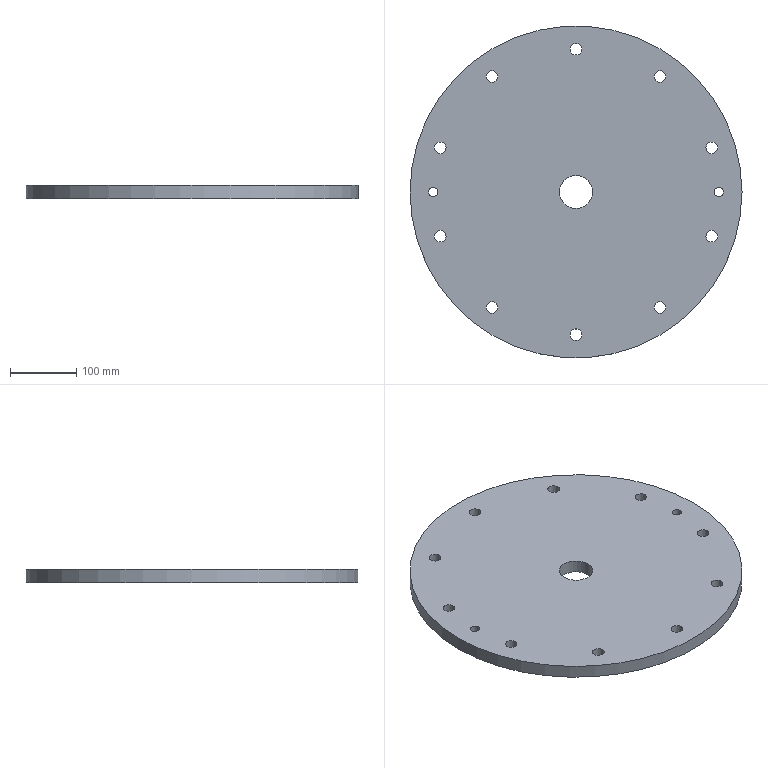NC program | NX | posted with a generic post | part box 500 x 500 x 20 mm
Whole program:
N10 G17 G21 G94 G90
(DRILLING , TOOL : ZXZ)
N12 T02 M6
N14 G54
N16 G17 G0 G90 X-126.374 Y-173.939 S3500 M3
N18 G43 Z30. H2
N20 G94 G81 G98 Z-2. F250. R3.
N22 X0. Y-215.
N24 X126.374 Y-173.939
N26 X204.477 Y-66.439
N28 X215. Y0.
N30 X204.477 Y66.439
N32 X126.374 Y173.939
N34 X0. Y215.
N36 X-126.374 Y173.939
N38 X-204.477 Y66.439
N40 X-215. Y0.
N42 X-204.477 Y-66.439
N44 G80
N46 G0 X-204.477 Y-66.439 Z30.
N48 M5
(DRILLING_COPY , TOOL : 17.5ZT)
N50 T17 M6
N52 G54
N54 G17 G0 G90 X0. Y-215. S500 M3
N56 G43 Z30. H17
N58 G94 G83 G98 Z-26.758 F100. Q2. R3.
N60 X-126.374 Y-173.939
N62 X-204.477 Y-66.439
N64 Y66.439
N66 X-126.374 Y173.939
N68 X0. Y215.
N70 X126.374 Y173.939
N72 X204.477 Y66.439
N74 Y-66.439
N76 X126.374 Y-173.939
N78 G80
N80 G0 X126.374 Y-173.939 Z30.
N82 M5
(DRILLING_COPY_COPY , TOOL : 14.0ZT)
N84 T14 M6
N86 G54
N88 G17 G0 G90 X215. Y0. S700 M3
N90 G43 Z30. H14
N92 G94 G83 G98 Z-25.706 F100. Q2. R3.
N94 X-215.
N96 G80
N98 G0 X-215. Y0. Z30.
N100 M5
N102 M2